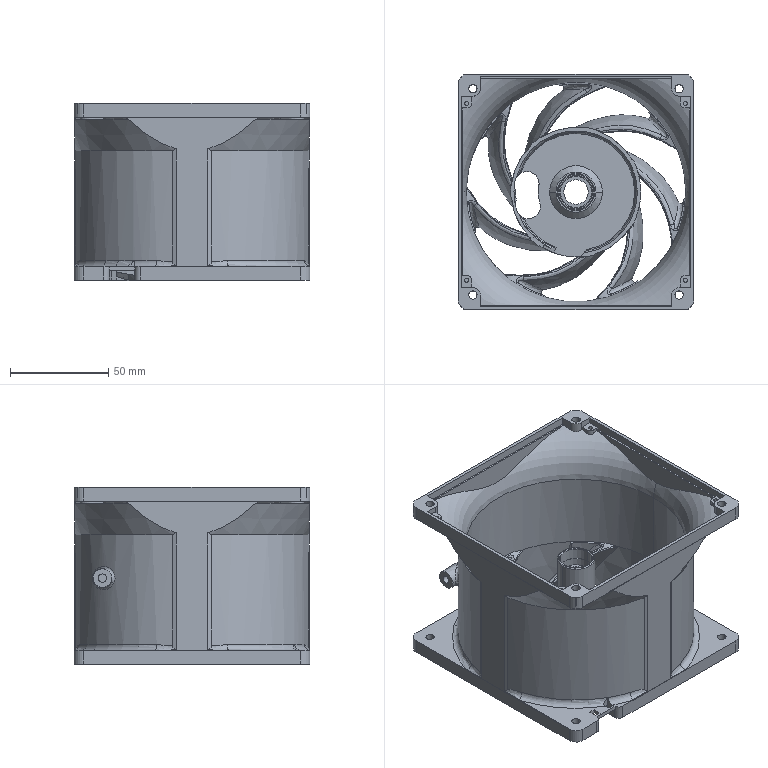NC program | NX | posted with a generic post | part box 120 x 120 x 90.2 mm
Lines 244469 to 245458 of 941997:
(型腔铣开粗铝料_COPY , TOOL : D4)
N488852 T05 M6
N488854 G54
N488856 G17 G0 G90 X-8.197 Y-26.183 S7500 M3
N488858 G43 Z49.153 H5
N488860 Z-1.1
N488862 G94 G1 X-8.217 Y-26.268 F2500.
N488864 X-8.268 Y-26.656
N488866 X-8.243 Y-27.048
N488868 X-8.142 Y-27.426
N488870 X-7.969 Y-27.778
N488872 X-7.731 Y-28.09
N488874 X-7.437 Y-28.349
N488876 X-7.097 Y-28.545
N488878 X-6.726 Y-28.672
N488880 X-6.452 Y-28.734
N488882 X-6.178 Y-28.795
N488884 X-5.641 Y-28.631
N488886 X-5.295 Y-28.488
N488888 X-4.982 Y-28.284
N488890 X-4.712 Y-28.025
N488892 X-4.495 Y-27.72
N488894 X-4.339 Y-27.38
N488896 X-4.249 Y-27.017
N488898 X-4.228 Y-26.643
N488900 X-4.277 Y-26.272
N488902 G0 Z2.153
N488904 X-8.197 Y-26.183
N488906 Z-1.475
N488908 G1 X-8.217 Y-26.268
N488910 X-8.268 Y-26.656
N488912 X-8.243 Y-27.048
N488914 X-8.142 Y-27.426
N488916 X-7.969 Y-27.778
N488918 X-7.731 Y-28.09
N488920 X-7.437 Y-28.349
N488922 X-7.097 Y-28.545
N488924 X-6.726 Y-28.672
N488926 X-6.452 Y-28.734
N488928 X-6.178 Y-28.795
N488930 X-5.641 Y-28.631
N488932 X-5.295 Y-28.488
N488934 X-4.982 Y-28.284
N488936 X-4.712 Y-28.025
N488938 X-4.495 Y-27.72
N488940 X-4.339 Y-27.38
N488942 X-4.249 Y-27.017
N488944 X-4.228 Y-26.643
N488946 X-4.277 Y-26.272
N488948 G0 Z1.9
N488950 X-8.197 Y-26.183
N488952 Z-1.85
N488954 G1 X-8.217 Y-26.268
N488956 X-8.268 Y-26.656
N488958 X-8.243 Y-27.048
N488960 X-8.142 Y-27.426
N488962 X-7.969 Y-27.778
N488964 X-7.731 Y-28.09
N488966 X-7.437 Y-28.349
N488968 X-7.097 Y-28.545
N488970 X-6.726 Y-28.672
N488972 X-6.452 Y-28.734
N488974 X-6.178 Y-28.795
N488976 X-5.641 Y-28.631
N488978 X-5.295 Y-28.488
N488980 X-4.982 Y-28.284
N488982 X-4.712 Y-28.025
N488984 X-4.495 Y-27.72
N488986 X-4.339 Y-27.38
N488988 X-4.249 Y-27.017
N488990 X-4.228 Y-26.643
N488992 X-4.277 Y-26.272
N488994 G0 Z1.525
N488996 X-8.197 Y-26.183
N488998 Z-2.225
N489000 G1 X-8.217 Y-26.268
N489002 X-8.268 Y-26.656
N489004 X-8.243 Y-27.048
N489006 X-8.142 Y-27.426
N489008 X-7.969 Y-27.778
N489010 X-7.731 Y-28.09
N489012 X-7.437 Y-28.349
N489014 X-7.097 Y-28.545
N489016 X-6.726 Y-28.672
N489018 X-6.452 Y-28.734
N489020 X-6.178 Y-28.795
N489022 X-5.641 Y-28.631
N489024 X-5.295 Y-28.488
N489026 X-4.982 Y-28.284
N489028 X-4.712 Y-28.025
N489030 X-4.495 Y-27.72
N489032 X-4.339 Y-27.38
N489034 X-4.249 Y-27.017
N489036 X-4.228 Y-26.643
N489038 X-4.277 Y-26.272
N489040 G0 Z1.15
N489042 X-8.197 Y-26.183
N489044 Z-2.6
N489046 G1 X-8.217 Y-26.268
N489048 X-8.268 Y-26.656
N489050 X-8.243 Y-27.048
N489052 X-8.142 Y-27.426
N489054 X-7.969 Y-27.778
N489056 X-7.731 Y-28.09
N489058 X-7.437 Y-28.349
N489060 X-7.097 Y-28.545
N489062 X-6.726 Y-28.672
N489064 X-6.452 Y-28.734
N489066 X-6.178 Y-28.795
N489068 X-5.641 Y-28.631
N489070 X-5.295 Y-28.488
N489072 X-4.982 Y-28.284
N489074 X-4.712 Y-28.025
N489076 X-4.495 Y-27.72
N489078 X-4.339 Y-27.38
N489080 X-4.249 Y-27.017
N489082 X-4.228 Y-26.643
N489084 X-4.277 Y-26.272
N489086 G0 Z0.775
N489088 X-8.197 Y-26.183
N489090 Z-2.975
N489092 G1 X-8.217 Y-26.268
N489094 X-8.268 Y-26.656
N489096 X-8.243 Y-27.048
N489098 X-8.142 Y-27.426
N489100 X-7.969 Y-27.778
N489102 X-7.731 Y-28.09
N489104 X-7.437 Y-28.349
N489106 X-7.097 Y-28.545
N489108 X-6.726 Y-28.672
N489110 X-6.452 Y-28.734
N489112 X-6.178 Y-28.795
N489114 X-5.641 Y-28.631
N489116 X-5.295 Y-28.488
N489118 X-4.982 Y-28.284
N489120 X-4.712 Y-28.025
N489122 X-4.495 Y-27.72
N489124 X-4.339 Y-27.38
N489126 X-4.249 Y-27.017
N489128 X-4.228 Y-26.643
N489130 X-4.277 Y-26.272
N489132 G0 Z0.4
N489134 X-8.197 Y-26.183
N489136 Z-3.35
N489138 G1 X-8.217 Y-26.268
N489140 X-8.268 Y-26.656
N489142 X-8.243 Y-27.048
N489144 X-8.142 Y-27.426
N489146 X-7.969 Y-27.778
N489148 X-7.731 Y-28.09
N489150 X-7.437 Y-28.349
N489152 X-7.097 Y-28.545
N489154 X-6.726 Y-28.672
N489156 X-6.452 Y-28.734
N489158 X-6.178 Y-28.795
N489160 X-5.641 Y-28.631
N489162 X-5.295 Y-28.488
N489164 X-4.982 Y-28.284
N489166 X-4.712 Y-28.025
N489168 X-4.495 Y-27.72
N489170 X-4.339 Y-27.38
N489172 X-4.249 Y-27.017
N489174 X-4.228 Y-26.643
N489176 X-4.277 Y-26.272
N489178 G0 Z0.025
N489180 X-8.197 Y-26.183
N489182 Z-3.725
N489184 G1 X-8.217 Y-26.268
N489186 X-8.268 Y-26.656
N489188 X-8.243 Y-27.048
N489190 X-8.142 Y-27.426
N489192 X-7.969 Y-27.778
N489194 X-7.731 Y-28.09
N489196 X-7.437 Y-28.349
N489198 X-7.097 Y-28.545
N489200 X-6.726 Y-28.672
N489202 X-6.452 Y-28.734
N489204 X-6.178 Y-28.795
N489206 X-5.641 Y-28.631
N489208 X-5.295 Y-28.488
N489210 X-4.982 Y-28.284
N489212 X-4.712 Y-28.025
N489214 X-4.495 Y-27.72
N489216 X-4.339 Y-27.38
N489218 X-4.249 Y-27.017
N489220 X-4.228 Y-26.643
N489222 X-4.277 Y-26.272
N489224 G0 Z-0.35
N489226 X-8.197 Y-26.183
N489228 Z-4.1
N489230 G1 X-8.217 Y-26.268
N489232 X-8.268 Y-26.656
N489234 X-8.243 Y-27.048
N489236 X-8.142 Y-27.426
N489238 X-7.969 Y-27.778
N489240 X-7.731 Y-28.09
N489242 X-7.437 Y-28.349
N489244 X-7.097 Y-28.545
N489246 X-6.726 Y-28.672
N489248 X-6.452 Y-28.734
N489250 X-6.178 Y-28.795
N489252 X-5.641 Y-28.631
N489254 X-5.295 Y-28.488
N489256 X-4.982 Y-28.284
N489258 X-4.712 Y-28.025
N489260 X-4.495 Y-27.72
N489262 X-4.339 Y-27.38
N489264 X-4.249 Y-27.017
N489266 X-4.228 Y-26.643
N489268 X-4.277 Y-26.272
N489270 G0 Z-0.725
N489272 X-8.197 Y-26.183
N489274 Z-4.5
N489276 G1 X-8.217 Y-26.268
N489278 X-8.268 Y-26.656
N489280 X-8.243 Y-27.048
N489282 X-8.142 Y-27.426
N489284 X-7.969 Y-27.778
N489286 X-7.731 Y-28.09
N489288 X-7.437 Y-28.349
N489290 X-7.097 Y-28.545
N489292 X-6.726 Y-28.672
N489294 X-6.452 Y-28.734
N489296 X-6.178 Y-28.795
N489298 X-5.641 Y-28.631
N489300 X-5.295 Y-28.488
N489302 X-4.982 Y-28.284
N489304 X-4.712 Y-28.025
N489306 X-4.495 Y-27.72
N489308 X-4.339 Y-27.38
N489310 X-4.249 Y-27.017
N489312 X-4.228 Y-26.643
N489314 X-4.277 Y-26.272
N489316 G0 Z-1.1
N489318 X-8.197 Y-26.183
N489320 Z-4.9
N489322 G1 X-8.217 Y-26.268
N489324 X-8.268 Y-26.656
N489326 X-8.243 Y-27.048
N489328 X-8.142 Y-27.426
N489330 X-7.969 Y-27.778
N489332 X-7.731 Y-28.09
N489334 X-7.437 Y-28.349
N489336 X-7.097 Y-28.545
N489338 X-6.726 Y-28.672
N489340 X-6.452 Y-28.734
N489342 X-6.178 Y-28.795
N489344 X-5.641 Y-28.631
N489346 X-5.295 Y-28.488
N489348 X-4.982 Y-28.284
N489350 X-4.712 Y-28.025
N489352 X-4.495 Y-27.72
N489354 X-4.339 Y-27.38
N489356 X-4.249 Y-27.017
N489358 X-4.228 Y-26.643
N489360 X-4.277 Y-26.272
N489362 G0 Z-1.5
N489364 X-8.197 Y-26.183
N489366 Z-5.3
N489368 G1 X-8.217 Y-26.268
N489370 X-8.268 Y-26.656
N489372 X-8.243 Y-27.048
N489374 X-8.142 Y-27.426
N489376 X-7.969 Y-27.778
N489378 X-7.731 Y-28.09
N489380 X-7.437 Y-28.349
N489382 X-7.097 Y-28.545
N489384 X-6.726 Y-28.672
N489386 X-6.452 Y-28.734
N489388 X-6.178 Y-28.795
N489390 X-5.641 Y-28.631
N489392 X-5.295 Y-28.488
N489394 X-4.982 Y-28.284
N489396 X-4.712 Y-28.025
N489398 X-4.495 Y-27.72
N489400 X-4.339 Y-27.38
N489402 X-4.249 Y-27.017
N489404 X-4.228 Y-26.643
N489406 X-4.277 Y-26.272
N489408 G0 Z-1.9
N489410 X-8.197 Y-26.183
N489412 Z-5.7
N489414 G1 X-8.217 Y-26.268
N489416 X-8.268 Y-26.656
N489418 X-8.243 Y-27.048
N489420 X-8.142 Y-27.426
N489422 X-7.969 Y-27.778
N489424 X-7.731 Y-28.09
N489426 X-7.437 Y-28.349
N489428 X-7.097 Y-28.545
N489430 X-6.726 Y-28.672
N489432 X-6.452 Y-28.734
N489434 X-6.178 Y-28.795
N489436 X-5.641 Y-28.631
N489438 X-5.295 Y-28.488
N489440 X-4.982 Y-28.284
N489442 X-4.712 Y-28.025
N489444 X-4.495 Y-27.72
N489446 X-4.339 Y-27.38
N489448 X-4.249 Y-27.017
N489450 X-4.228 Y-26.643
N489452 X-4.277 Y-26.272
N489454 G0 Z-2.3
N489456 X-8.197 Y-26.183
N489458 Z-6.1
N489460 G1 X-8.217 Y-26.268
N489462 X-8.268 Y-26.656
N489464 X-8.243 Y-27.048
N489466 X-8.142 Y-27.426
N489468 X-7.969 Y-27.778
N489470 X-7.731 Y-28.09
N489472 X-7.437 Y-28.349
N489474 X-7.097 Y-28.545
N489476 X-6.726 Y-28.672
N489478 X-6.452 Y-28.734
N489480 X-6.178 Y-28.795
N489482 X-5.641 Y-28.631
N489484 X-5.295 Y-28.488
N489486 X-4.982 Y-28.284
N489488 X-4.712 Y-28.025
N489490 X-4.495 Y-27.72
N489492 X-4.339 Y-27.38
N489494 X-4.249 Y-27.017
N489496 X-4.228 Y-26.643
N489498 X-4.277 Y-26.272
N489500 G0 Z-2.7
N489502 X-8.197 Y-26.183
N489504 Z-6.485
N489506 G1 X-8.217 Y-26.268
N489508 X-8.268 Y-26.656
N489510 X-8.243 Y-27.048
N489512 X-8.142 Y-27.426
N489514 X-7.969 Y-27.778
N489516 X-7.731 Y-28.09
N489518 X-7.437 Y-28.349
N489520 X-7.097 Y-28.545
N489522 X-6.726 Y-28.672
N489524 X-6.452 Y-28.734
N489526 X-6.178 Y-28.795
N489528 X-5.641 Y-28.631
N489530 X-5.295 Y-28.488
N489532 X-4.982 Y-28.284
N489534 X-4.712 Y-28.025
N489536 X-4.495 Y-27.72
N489538 X-4.339 Y-27.38
N489540 X-4.249 Y-27.017
N489542 X-4.228 Y-26.643
N489544 X-4.277 Y-26.272
N489546 G0 Z-3.1
N489548 X-8.197 Y-26.183
N489550 Z-6.869
N489552 G1 X-8.217 Y-26.268
N489554 X-8.268 Y-26.656
N489556 X-8.243 Y-27.048
N489558 X-8.142 Y-27.426
N489560 X-7.969 Y-27.778
N489562 X-7.731 Y-28.09
N489564 X-7.437 Y-28.349
N489566 X-7.097 Y-28.545
N489568 X-6.726 Y-28.672
N489570 X-6.452 Y-28.734
N489572 X-6.178 Y-28.795
N489574 X-5.641 Y-28.631
N489576 X-5.295 Y-28.488
N489578 X-4.982 Y-28.284
N489580 X-4.712 Y-28.025
N489582 X-4.495 Y-27.72
N489584 X-4.339 Y-27.38
N489586 X-4.249 Y-27.017
N489588 X-4.228 Y-26.643
N489590 X-4.277 Y-26.272
N489592 G0 Z-3.485
N489594 X-8.197 Y-26.183
N489596 Z-7.254
N489598 G1 X-8.217 Y-26.268
N489600 X-8.268 Y-26.656
N489602 X-8.243 Y-27.048
N489604 X-8.142 Y-27.426
N489606 X-7.969 Y-27.778
N489608 X-7.731 Y-28.09
N489610 X-7.437 Y-28.349
N489612 X-7.097 Y-28.545
N489614 X-6.726 Y-28.672
N489616 X-6.452 Y-28.734
N489618 X-6.178 Y-28.795
N489620 X-5.641 Y-28.631
N489622 X-5.295 Y-28.488
N489624 X-4.982 Y-28.284
N489626 X-4.712 Y-28.025
N489628 X-4.495 Y-27.72
N489630 X-4.339 Y-27.38
N489632 X-4.249 Y-27.017
N489634 X-4.228 Y-26.643
N489636 X-4.277 Y-26.272
N489638 G0 Z-3.869
N489640 X-8.197 Y-26.183
N489642 Z-7.638
N489644 G1 X-8.217 Y-26.268
N489646 X-8.268 Y-26.656
N489648 X-8.243 Y-27.048
N489650 X-8.142 Y-27.426
N489652 X-7.969 Y-27.778
N489654 X-7.731 Y-28.09
N489656 X-7.437 Y-28.349
N489658 X-7.097 Y-28.545
N489660 X-6.726 Y-28.672
N489662 X-6.452 Y-28.734
N489664 X-6.178 Y-28.795
N489666 X-5.641 Y-28.631
N489668 X-5.295 Y-28.488
N489670 X-4.982 Y-28.284
N489672 X-4.712 Y-28.025
N489674 X-4.495 Y-27.72
N489676 X-4.339 Y-27.38
N489678 X-4.249 Y-27.017
N489680 X-4.228 Y-26.643
N489682 X-4.277 Y-26.272
N489684 G0 Z-4.254
N489686 X-8.197 Y-26.183
N489688 Z-8.023
N489690 G1 X-8.217 Y-26.268
N489692 X-8.268 Y-26.656
N489694 X-8.243 Y-27.048
N489696 X-8.142 Y-27.426
N489698 X-7.969 Y-27.778
N489700 X-7.731 Y-28.09
N489702 X-7.437 Y-28.349
N489704 X-7.097 Y-28.545
N489706 X-6.726 Y-28.672
N489708 X-6.452 Y-28.734
N489710 X-6.178 Y-28.795
N489712 X-5.641 Y-28.631
N489714 X-5.295 Y-28.488
N489716 X-4.982 Y-28.284
N489718 X-4.712 Y-28.025
N489720 X-4.495 Y-27.72
N489722 X-4.339 Y-27.38
N489724 X-4.249 Y-27.017
N489726 X-4.228 Y-26.643
N489728 X-4.277 Y-26.272
N489730 G0 Z-4.638
N489732 X-8.196 Y-26.184
N489734 Z-8.408
N489736 G1 X-8.215 Y-26.268
N489738 X-8.267 Y-26.657
N489740 X-8.242 Y-27.048
N489742 X-8.141 Y-27.427
N489744 X-7.968 Y-27.779
N489746 X-7.73 Y-28.09
N489748 X-7.435 Y-28.349
N489750 X-7.096 Y-28.545
N489752 X-6.725 Y-28.672
N489754 X-6.637 Y-28.692
N489756 X-6.55 Y-28.712
N489758 X-6.178 Y-28.795
N489760 X-5.641 Y-28.631
N489762 X-5.295 Y-28.488
N489764 X-4.982 Y-28.284
N489766 X-4.712 Y-28.025
N489768 X-4.495 Y-27.72
N489770 X-4.339 Y-27.38
N489772 X-4.249 Y-27.017
N489774 X-4.228 Y-26.643
N489776 X-4.277 Y-26.272
N489778 G0 Z-5.023
N489780 X-8.191 Y-26.186
N489782 Z-8.792
N489784 G1 X-8.21 Y-26.27
N489786 X-8.262 Y-26.658
N489788 X-8.237 Y-27.05
N489790 X-8.136 Y-27.428
N489792 X-7.963 Y-27.78
N489794 X-7.724 Y-28.092
N489796 X-7.43 Y-28.35
N489798 X-7.09 Y-28.547
N489800 X-6.719 Y-28.673
N489802 X-6.635 Y-28.693
N489804 X-6.55 Y-28.712
N489806 X-6.178 Y-28.795
N489808 X-5.649 Y-28.633
N489810 X-5.303 Y-28.491
N489812 X-4.989 Y-28.286
N489814 X-4.719 Y-28.027
N489816 X-4.503 Y-27.721
N489818 X-4.346 Y-27.381
N489820 X-4.256 Y-27.017
N489822 X-4.236 Y-26.643
N489824 X-4.285 Y-26.272
N489826 G0 Z-5.408
N489828 X-8.191 Y-26.186
N489830 Z-9.177
N489832 G1 X-8.21 Y-26.27
N489834 X-8.262 Y-26.658
N489836 X-8.237 Y-27.05
N489838 X-8.136 Y-27.428
N489840 X-7.963 Y-27.78
N489842 X-7.724 Y-28.092
N489844 X-7.43 Y-28.35
N489846 X-7.09 Y-28.547
N489848 X-6.719 Y-28.673
N489850 X-6.635 Y-28.693
N489852 X-6.55 Y-28.712
N489854 X-6.178 Y-28.795
N489856 X-5.649 Y-28.633
N489858 X-5.303 Y-28.491
N489860 X-4.989 Y-28.286
N489862 X-4.719 Y-28.027
N489864 X-4.503 Y-27.721
N489866 X-4.346 Y-27.381
N489868 X-4.256 Y-27.017
N489870 X-4.236 Y-26.643
N489872 X-4.285 Y-26.272
N489874 G0 Z-5.792
N489876 X-8.191 Y-26.186
N489878 Z-9.562
N489880 G1 X-8.21 Y-26.27
N489882 X-8.262 Y-26.658
N489884 X-8.237 Y-27.05
N489886 X-8.136 Y-27.428
N489888 X-7.963 Y-27.78
N489890 X-7.724 Y-28.092
N489892 X-7.43 Y-28.35
N489894 X-7.09 Y-28.547
N489896 X-6.719 Y-28.673
N489898 X-6.635 Y-28.693
N489900 X-6.55 Y-28.712
N489902 X-6.178 Y-28.795
N489904 X-5.649 Y-28.633
N489906 X-5.303 Y-28.491
N489908 X-4.989 Y-28.286
N489910 X-4.719 Y-28.027
N489912 X-4.503 Y-27.721
N489914 X-4.346 Y-27.381
N489916 X-4.256 Y-27.017
N489918 X-4.236 Y-26.643
N489920 X-4.285 Y-26.272
N489922 G0 Z-6.177
N489924 X-8.191 Y-26.186
N489926 Z-9.946
N489928 G1 X-8.21 Y-26.27
N489930 X-8.262 Y-26.658
N489932 X-8.237 Y-27.05
N489934 X-8.136 Y-27.428
N489936 X-7.963 Y-27.78
N489938 X-7.724 Y-28.092
N489940 X-7.43 Y-28.35
N489942 X-7.09 Y-28.547
N489944 X-6.719 Y-28.673
N489946 X-6.635 Y-28.693
N489948 X-6.55 Y-28.712
N489950 X-6.178 Y-28.795
N489952 X-5.649 Y-28.633
N489954 X-5.303 Y-28.491
N489956 X-4.989 Y-28.286
N489958 X-4.719 Y-28.027
N489960 X-4.503 Y-27.721
N489962 X-4.346 Y-27.381
N489964 X-4.256 Y-27.017
N489966 X-4.236 Y-26.643
N489968 X-4.285 Y-26.272
N489970 G0 Z-6.562
N489972 X-8.191 Y-26.186
N489974 Z-10.331
N489976 G1 X-8.21 Y-26.27
N489978 X-8.262 Y-26.658
N489980 X-8.237 Y-27.05
N489982 X-8.136 Y-27.428
N489984 X-7.963 Y-27.78
N489986 X-7.724 Y-28.092
N489988 X-7.43 Y-28.35
N489990 X-7.09 Y-28.547
N489992 X-6.719 Y-28.673
N489994 X-6.635 Y-28.693
N489996 X-6.55 Y-28.712
N489998 X-6.178 Y-28.795
N490000 X-5.649 Y-28.633
N490002 X-5.303 Y-28.491
N490004 X-4.989 Y-28.286
N490006 X-4.719 Y-28.027
N490008 X-4.503 Y-27.721
N490010 X-4.346 Y-27.381
N490012 X-4.256 Y-27.017
N490014 X-4.236 Y-26.643
N490016 X-4.285 Y-26.272
N490018 G0 Z-6.946
N490020 X-8.191 Y-26.186
N490022 Z-10.715
N490024 G1 X-8.21 Y-26.27
N490026 X-8.262 Y-26.658
N490028 X-8.237 Y-27.05
N490030 X-8.136 Y-27.428
N490032 X-7.963 Y-27.78
N490034 X-7.724 Y-28.092
N490036 X-7.43 Y-28.35
N490038 X-7.09 Y-28.547
N490040 X-6.719 Y-28.673
N490042 X-6.635 Y-28.693
N490044 X-6.55 Y-28.712
N490046 X-6.178 Y-28.795
N490048 X-5.649 Y-28.633
N490050 X-5.303 Y-28.491
N490052 X-4.989 Y-28.286
N490054 X-4.719 Y-28.027
N490056 X-4.503 Y-27.721
N490058 X-4.346 Y-27.381
N490060 X-4.256 Y-27.017
N490062 X-4.236 Y-26.643
N490064 X-4.285 Y-26.272
N490066 G0 Z-7.331
N490068 X-8.191 Y-26.186
N490070 Z-11.1
N490072 G1 X-8.21 Y-26.27
N490074 X-8.262 Y-26.658
N490076 X-8.237 Y-27.05
N490078 X-8.136 Y-27.428
N490080 X-7.963 Y-27.78
N490082 X-7.724 Y-28.092
N490084 X-7.43 Y-28.35
N490086 X-7.09 Y-28.547
N490088 X-6.719 Y-28.673
N490090 X-6.635 Y-28.693
N490092 X-6.55 Y-28.712
N490094 X-6.178 Y-28.795
N490096 X-5.649 Y-28.633
N490098 X-5.303 Y-28.491
N490100 X-4.989 Y-28.286
N490102 X-4.719 Y-28.027
N490104 X-4.503 Y-27.721
N490106 X-4.346 Y-27.381
N490108 X-4.256 Y-27.017
N490110 X-4.236 Y-26.643
N490112 X-4.285 Y-26.272
N490114 G0 Z-7.715
N490116 X-8.191 Y-26.186
N490118 Z-11.491
N490120 G1 X-8.21 Y-26.27
N490122 X-8.262 Y-26.658
N490124 X-8.237 Y-27.05
N490126 X-8.136 Y-27.428
N490128 X-7.963 Y-27.78
N490130 X-7.724 Y-28.092
N490132 X-7.43 Y-28.35
N490134 X-7.09 Y-28.547
N490136 X-6.719 Y-28.673
N490138 X-6.635 Y-28.693
N490140 X-6.55 Y-28.712
N490142 X-6.178 Y-28.795
N490144 X-5.649 Y-28.633
N490146 X-5.303 Y-28.491
N490148 X-4.989 Y-28.286
N490150 X-4.719 Y-28.027
N490152 X-4.503 Y-27.721
N490154 X-4.346 Y-27.381
N490156 X-4.256 Y-27.017
N490158 X-4.236 Y-26.643
N490160 X-4.285 Y-26.272
N490162 G0 Z-8.1
N490164 X-8.191 Y-26.186
N490166 Z-11.882
N490168 G1 X-8.21 Y-26.27
N490170 X-8.262 Y-26.658
N490172 X-8.237 Y-27.05
N490174 X-8.136 Y-27.428
N490176 X-7.963 Y-27.78
N490178 X-7.724 Y-28.092
N490180 X-7.43 Y-28.35
N490182 X-7.09 Y-28.547
N490184 X-6.719 Y-28.673
N490186 X-6.635 Y-28.693
N490188 X-6.55 Y-28.712
N490190 X-6.178 Y-28.795
N490192 X-5.649 Y-28.633
N490194 X-5.303 Y-28.491
N490196 X-4.989 Y-28.286
N490198 X-4.719 Y-28.027
N490200 X-4.503 Y-27.721
N490202 X-4.346 Y-27.381
N490204 X-4.256 Y-27.017
N490206 X-4.236 Y-26.643
N490208 X-4.285 Y-26.272
N490210 G0 Z-8.491
N490212 X-8.191 Y-26.186
N490214 Z-12.273
N490216 G1 X-8.21 Y-26.27
N490218 X-8.262 Y-26.658
N490220 X-8.237 Y-27.05
N490222 X-8.136 Y-27.428
N490224 X-7.963 Y-27.78
N490226 X-7.724 Y-28.092
N490228 X-7.43 Y-28.35
N490230 X-7.09 Y-28.547
N490232 X-6.719 Y-28.673
N490234 X-6.635 Y-28.693
N490236 X-6.55 Y-28.712
N490238 X-6.178 Y-28.795
N490240 X-5.649 Y-28.633
N490242 X-5.303 Y-28.491
N490244 X-4.989 Y-28.286
N490246 X-4.719 Y-28.027
N490248 X-4.503 Y-27.721
N490250 X-4.346 Y-27.381
N490252 X-4.256 Y-27.017
N490254 X-4.236 Y-26.643
N490256 X-4.285 Y-26.272
N490258 G0 Z-8.882
N490260 X-8.191 Y-26.186
N490262 Z-12.664
N490264 G1 X-8.21 Y-26.27
N490266 X-8.262 Y-26.658
N490268 X-8.237 Y-27.05
N490270 X-8.136 Y-27.428
N490272 X-7.963 Y-27.78
N490274 X-7.724 Y-28.092
N490276 X-7.43 Y-28.35
N490278 X-7.09 Y-28.547
N490280 X-6.719 Y-28.673
N490282 X-6.635 Y-28.693
N490284 X-6.55 Y-28.712
N490286 X-6.178 Y-28.795
N490288 X-5.649 Y-28.633
N490290 X-5.303 Y-28.491
N490292 X-4.989 Y-28.286
N490294 X-4.719 Y-28.027
N490296 X-4.503 Y-27.721
N490298 X-4.346 Y-27.381
N490300 X-4.256 Y-27.017
N490302 X-4.236 Y-26.643
N490304 X-4.285 Y-26.272
N490306 G0 Z-9.273
N490308 X-8.199 Y-26.182
N490310 Z-13.055
N490312 G1 X-8.219 Y-26.267
N490314 X-8.271 Y-26.656
N490316 X-8.246 Y-27.047
N490318 X-8.145 Y-27.426
N490320 X-7.972 Y-27.778
N490322 X-7.733 Y-28.089
N490324 X-7.439 Y-28.348
N490326 X-7.1 Y-28.544
N490328 X-6.729 Y-28.671
N490330 X-6.639 Y-28.692
N490332 X-6.55 Y-28.712
N490334 X-6.178 Y-28.795
N490336 X-5.635 Y-28.629
N490338 X-5.289 Y-28.486
N490340 X-4.976 Y-28.282
N490342 X-4.706 Y-28.023
N490344 X-4.489 Y-27.719
N490346 X-4.333 Y-27.379
N490348 X-4.242 Y-27.016
N490350 X-4.221 Y-26.643
N490352 X-4.27 Y-26.272
N490354 G0 Z-9.664
N490356 X-8.199 Y-26.182
N490358 Z-13.445
N490360 G1 X-8.219 Y-26.267
N490362 X-8.271 Y-26.656
N490364 X-8.246 Y-27.047
N490366 X-8.145 Y-27.426
N490368 X-7.972 Y-27.778
N490370 X-7.733 Y-28.089
N490372 X-7.439 Y-28.348
N490374 X-7.1 Y-28.544
N490376 X-6.729 Y-28.671
N490378 X-6.639 Y-28.692
N490380 X-6.55 Y-28.712
N490382 X-6.178 Y-28.795
N490384 X-5.635 Y-28.629
N490386 X-5.289 Y-28.486
N490388 X-4.976 Y-28.282
N490390 X-4.706 Y-28.023
N490392 X-4.489 Y-27.719
N490394 X-4.333 Y-27.379
N490396 X-4.242 Y-27.016
N490398 X-4.221 Y-26.643
N490400 X-4.27 Y-26.272
N490402 G0 Z-10.055
N490404 X-8.199 Y-26.182
N490406 Z-13.836
N490408 G1 X-8.219 Y-26.267
N490410 X-8.271 Y-26.656
N490412 X-8.246 Y-27.047
N490414 X-8.145 Y-27.426
N490416 X-7.972 Y-27.778
N490418 X-7.733 Y-28.089
N490420 X-7.439 Y-28.348
N490422 X-7.1 Y-28.544
N490424 X-6.729 Y-28.671
N490426 X-6.639 Y-28.692
N490428 X-6.55 Y-28.712
N490430 X-6.178 Y-28.795
N490432 X-5.635 Y-28.629
N490434 X-5.289 Y-28.486
N490436 X-4.976 Y-28.282
N490438 X-4.706 Y-28.023
N490440 X-4.489 Y-27.719
N490442 X-4.333 Y-27.379
N490444 X-4.242 Y-27.016
N490446 X-4.221 Y-26.643
N490448 X-4.27 Y-26.272
N490450 G0 Z-10.445
N490452 X-8.199 Y-26.182
N490454 Z-14.227
N490456 G1 X-8.219 Y-26.267
N490458 X-8.271 Y-26.656
N490460 X-8.246 Y-27.047
N490462 X-8.145 Y-27.426
N490464 X-7.972 Y-27.778
N490466 X-7.733 Y-28.089
N490468 X-7.439 Y-28.348
N490470 X-7.1 Y-28.544
N490472 X-6.729 Y-28.671
N490474 X-6.639 Y-28.692
N490476 X-6.55 Y-28.712
N490478 X-6.178 Y-28.795
N490480 X-5.635 Y-28.629
N490482 X-5.289 Y-28.486
N490484 X-4.976 Y-28.282
N490486 X-4.706 Y-28.023
N490488 X-4.489 Y-27.719
N490490 X-4.333 Y-27.379
N490492 X-4.242 Y-27.016
N490494 X-4.221 Y-26.643
N490496 X-4.27 Y-26.272
N490498 G0 Z-10.836
N490500 X-8.199 Y-26.182
N490502 Z-14.618
N490504 G1 X-8.219 Y-26.267
N490506 X-8.271 Y-26.656
N490508 X-8.246 Y-27.047
N490510 X-8.145 Y-27.426
N490512 X-7.972 Y-27.778
N490514 X-7.733 Y-28.089
N490516 X-7.439 Y-28.348
N490518 X-7.1 Y-28.544
N490520 X-6.729 Y-28.671
N490522 X-6.639 Y-28.692
N490524 X-6.55 Y-28.712
N490526 X-6.178 Y-28.795
N490528 X-5.635 Y-28.629
N490530 X-5.289 Y-28.486
N490532 X-4.976 Y-28.282
N490534 X-4.706 Y-28.023
N490536 X-4.489 Y-27.719
N490538 X-4.333 Y-27.379
N490540 X-4.242 Y-27.016
N490542 X-4.221 Y-26.643
N490544 X-4.27 Y-26.272
N490546 G0 Z-11.227
N490548 X-8.199 Y-26.182
N490550 Z-15.009
N490552 G1 X-8.219 Y-26.267
N490554 X-8.271 Y-26.656
N490556 X-8.246 Y-27.047
N490558 X-8.145 Y-27.426
N490560 X-7.972 Y-27.778
N490562 X-7.733 Y-28.089
N490564 X-7.439 Y-28.348
N490566 X-7.1 Y-28.544
N490568 X-6.729 Y-28.671
N490570 X-6.639 Y-28.692
N490572 X-6.55 Y-28.712
N490574 X-6.178 Y-28.795
N490576 X-5.635 Y-28.629
N490578 X-5.289 Y-28.486
N490580 X-4.976 Y-28.282
N490582 X-4.706 Y-28.023
N490584 X-4.489 Y-27.719
N490586 X-4.333 Y-27.379
N490588 X-4.242 Y-27.016
N490590 X-4.221 Y-26.643
N490592 X-4.27 Y-26.272
N490594 G0 Z-11.618
N490596 X-8.199 Y-26.182
N490598 Z-15.4
N490600 G1 X-8.219 Y-26.267
N490602 X-8.271 Y-26.656
N490604 X-8.246 Y-27.047
N490606 X-8.145 Y-27.426
N490608 X-7.972 Y-27.778
N490610 X-7.733 Y-28.089
N490612 X-7.439 Y-28.348
N490614 X-7.1 Y-28.544
N490616 X-6.729 Y-28.671
N490618 X-6.639 Y-28.692
N490620 X-6.55 Y-28.712
N490622 X-6.178 Y-28.795
N490624 X-5.635 Y-28.629
N490626 X-5.289 Y-28.486
N490628 X-4.976 Y-28.282
N490630 X-4.706 Y-28.023
N490632 X-4.489 Y-27.719
N490634 X-4.333 Y-27.379
N490636 X-4.242 Y-27.016
N490638 X-4.221 Y-26.643
N490640 X-4.27 Y-26.272
N490642 G0 Z-12.009
N490644 X-8.199 Y-26.182
N490646 Z-15.791
N490648 G1 X-8.219 Y-26.267
N490650 X-8.271 Y-26.656
N490652 X-8.246 Y-27.047
N490654 X-8.145 Y-27.426
N490656 X-7.972 Y-27.778
N490658 X-7.733 Y-28.089
N490660 X-7.439 Y-28.348
N490662 X-7.1 Y-28.544
N490664 X-6.729 Y-28.671
N490666 X-6.639 Y-28.692
N490668 X-6.55 Y-28.712
N490670 X-6.178 Y-28.795
N490672 X-5.635 Y-28.629
N490674 X-5.289 Y-28.486
N490676 X-4.976 Y-28.282
N490678 X-4.706 Y-28.023
N490680 X-4.489 Y-27.719
N490682 X-4.333 Y-27.379
N490684 X-4.242 Y-27.016
N490686 X-4.221 Y-26.643
N490688 X-4.27 Y-26.272
N490690 G0 Z-12.4
N490692 X-8.199 Y-26.182
N490694 Z-16.182
N490696 G1 X-8.219 Y-26.267
N490698 X-8.271 Y-26.656
N490700 X-8.246 Y-27.047
N490702 X-8.145 Y-27.426
N490704 X-7.972 Y-27.778
N490706 X-7.733 Y-28.089
N490708 X-7.439 Y-28.348
N490710 X-7.1 Y-28.544
N490712 X-6.729 Y-28.671
N490714 X-6.639 Y-28.692
N490716 X-6.55 Y-28.712
N490718 X-6.178 Y-28.795
N490720 X-5.635 Y-28.629
N490722 X-5.289 Y-28.486
N490724 X-4.976 Y-28.282
N490726 X-4.706 Y-28.023
N490728 X-4.489 Y-27.719
N490730 X-4.333 Y-27.379
N490732 X-4.242 Y-27.016
N490734 X-4.221 Y-26.643
N490736 X-4.27 Y-26.272
N490738 G0 Z-12.791
N490740 X-8.199 Y-26.182
N490742 Z-16.573
N490744 G1 X-8.219 Y-26.267
N490746 X-8.271 Y-26.656
N490748 X-8.246 Y-27.047
N490750 X-8.145 Y-27.426
N490752 X-7.972 Y-27.778
N490754 X-7.733 Y-28.089
N490756 X-7.439 Y-28.348
N490758 X-7.1 Y-28.544
N490760 X-6.729 Y-28.671
N490762 X-6.639 Y-28.692
N490764 X-6.55 Y-28.712
N490766 X-6.178 Y-28.795
N490768 X-5.635 Y-28.629
N490770 X-5.289 Y-28.486
N490772 X-4.976 Y-28.282
N490774 X-4.706 Y-28.023
N490776 X-4.489 Y-27.719
N490778 X-4.333 Y-27.379
N490780 X-4.242 Y-27.016
N490782 X-4.221 Y-26.643
N490784 X-4.27 Y-26.272
N490786 G0 Z-13.182
N490788 X-8.199 Y-26.182
N490790 Z-16.964
N490792 G1 X-8.219 Y-26.267
N490794 X-8.271 Y-26.656
N490796 X-8.246 Y-27.047
N490798 X-8.145 Y-27.426
N490800 X-7.972 Y-27.778
N490802 X-7.733 Y-28.089
N490804 X-7.439 Y-28.348
N490806 X-7.1 Y-28.544
N490808 X-6.729 Y-28.671
N490810 X-6.639 Y-28.692
N490812 X-6.55 Y-28.712
N490814 X-6.178 Y-28.795
N490816 X-5.635 Y-28.629
N490818 X-5.289 Y-28.486
N490820 X-4.976 Y-28.282
N490822 X-4.706 Y-28.023
N490824 X-4.489 Y-27.719